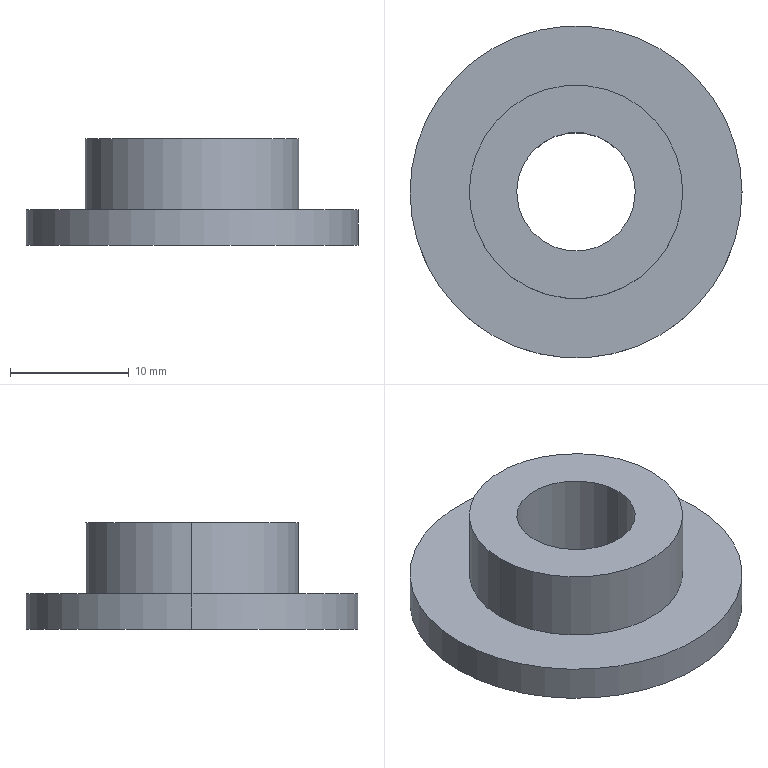Part | SolidWorks | features ICE 2, Extrusion 1 | 1 solid | 9 faces | box 28 x 28 x 9 mm | volume 2667 mm3 | cylinder 6 | plane 3 | commonest cylinder face diameters 10 x2 18 x2 28 x2
STEP:
#1=CARTESIAN_POINT('',(-5.,0.,0.));
#2=VERTEX_POINT('',#1);
#3=CARTESIAN_POINT('',(5.,0.,0.));
#4=VERTEX_POINT('',#3);
#5=CARTESIAN_POINT('',(0.,0.,0.));
#6=DIRECTION('',(0.,0.,1.));
#7=DIRECTION('',(1.,0.,0.));
#8=AXIS2_PLACEMENT_3D('',#5,#6,#7);
#9=CIRCLE('',#8,5.);
#10=EDGE_CURVE('',#2,#4,#9,.T.);
#11=ORIENTED_EDGE('',*,*,#10,.F.);
#12=CARTESIAN_POINT('',(-5.,0.,9.));
#13=VERTEX_POINT('',#12);
#14=CARTESIAN_POINT('',(-5.,0.,-3.));
#15=DIRECTION('',(0.,0.,1.));
#16=VECTOR('',#15,1000.);
#17=LINE('',#14,#16);
#18=EDGE_CURVE('',#2,#13,#17,.T.);
#19=ORIENTED_EDGE('',*,*,#18,.T.);
#20=CARTESIAN_POINT('',(5.,0.,9.));
#21=VERTEX_POINT('',#20);
#22=CARTESIAN_POINT('',(0.,0.,9.));
#23=DIRECTION('',(0.,0.,1.));
#24=DIRECTION('',(1.,0.,0.));
#25=AXIS2_PLACEMENT_3D('',#22,#23,#24);
#26=CIRCLE('',#25,5.);
#27=EDGE_CURVE('',#13,#21,#26,.T.);
#28=ORIENTED_EDGE('',*,*,#27,.T.);
#29=CARTESIAN_POINT('',(5.,0.,-3.));
#30=DIRECTION('',(0.,0.,1.));
#31=VECTOR('',#30,1000.);
#32=LINE('',#29,#31);
#33=EDGE_CURVE('',#4,#21,#32,.T.);
#34=ORIENTED_EDGE('',*,*,#33,.F.);
#35=EDGE_LOOP('',(#11,#19,#28,#34));
#36=FACE_OUTER_BOUND('',#35,.T.);
#37=CARTESIAN_POINT('',(0.,0.,-3.));
#38=DIRECTION('',(0.,0.,1.));
#39=DIRECTION('',(1.,0.,0.));
#40=AXIS2_PLACEMENT_3D('',#37,#38,#39);
#41=CYLINDRICAL_SURFACE('',#40,5.);
#42=ADVANCED_FACE('',(#36),#41,.F.);
#43=CARTESIAN_POINT('',(9.,0.,9.));
#44=VERTEX_POINT('',#43);
#45=CARTESIAN_POINT('',(-9.,0.,9.));
#46=VERTEX_POINT('',#45);
#47=CARTESIAN_POINT('',(0.,0.,9.));
#48=DIRECTION('',(0.,0.,1.));
#49=DIRECTION('',(1.,0.,0.));
#50=AXIS2_PLACEMENT_3D('',#47,#48,#49);
#51=CIRCLE('',#50,9.);
#52=EDGE_CURVE('',#44,#46,#51,.T.);
#53=ORIENTED_EDGE('',*,*,#52,.F.);
#54=CARTESIAN_POINT('',(9.,0.,3.));
#55=VERTEX_POINT('',#54);
#56=CARTESIAN_POINT('',(9.,0.,9.));
#57=DIRECTION('',(0.,0.,-1.));
#58=VECTOR('',#57,1000.);
#59=LINE('',#56,#58);
#60=EDGE_CURVE('',#44,#55,#59,.T.);
#61=ORIENTED_EDGE('',*,*,#60,.T.);
#62=CARTESIAN_POINT('',(-9.,0.,3.));
#63=VERTEX_POINT('',#62);
#64=CARTESIAN_POINT('',(0.,0.,3.));
#65=DIRECTION('',(0.,0.,1.));
#66=DIRECTION('',(1.,0.,0.));
#67=AXIS2_PLACEMENT_3D('',#64,#65,#66);
#68=CIRCLE('',#67,9.);
#69=EDGE_CURVE('',#55,#63,#68,.T.);
#70=ORIENTED_EDGE('',*,*,#69,.T.);
#71=CARTESIAN_POINT('',(-9.,0.,9.));
#72=DIRECTION('',(0.,0.,-1.));
#73=VECTOR('',#72,1000.);
#74=LINE('',#71,#73);
#75=EDGE_CURVE('',#46,#63,#74,.T.);
#76=ORIENTED_EDGE('',*,*,#75,.F.);
#77=EDGE_LOOP('',(#53,#61,#70,#76));
#78=FACE_OUTER_BOUND('',#77,.T.);
#79=CARTESIAN_POINT('',(0.,0.,9.));
#80=DIRECTION('',(0.,0.,-1.));
#81=DIRECTION('',(-1.,0.,0.));
#82=AXIS2_PLACEMENT_3D('',#79,#80,#81);
#83=CYLINDRICAL_SURFACE('',#82,9.);
#84=ADVANCED_FACE('',(#78),#83,.T.);
#85=CARTESIAN_POINT('',(14.,0.,3.));
#86=VERTEX_POINT('',#85);
#87=CARTESIAN_POINT('',(-14.,0.,3.));
#88=VERTEX_POINT('',#87);
#89=CARTESIAN_POINT('',(0.,0.,3.));
#90=DIRECTION('',(0.,0.,1.));
#91=DIRECTION('',(1.,0.,0.));
#92=AXIS2_PLACEMENT_3D('',#89,#90,#91);
#93=CIRCLE('',#92,14.);
#94=EDGE_CURVE('',#86,#88,#93,.T.);
#95=ORIENTED_EDGE('',*,*,#94,.F.);
#96=CARTESIAN_POINT('',(14.,0.,0.));
#97=VERTEX_POINT('',#96);
#98=CARTESIAN_POINT('',(14.,0.,3.));
#99=DIRECTION('',(0.,0.,-1.));
#100=VECTOR('',#99,1000.);
#101=LINE('',#98,#100);
#102=EDGE_CURVE('',#86,#97,#101,.T.);
#103=ORIENTED_EDGE('',*,*,#102,.T.);
#104=CARTESIAN_POINT('',(-14.,0.,0.));
#105=VERTEX_POINT('',#104);
#106=CARTESIAN_POINT('',(0.,0.,0.));
#107=DIRECTION('',(0.,0.,1.));
#108=DIRECTION('',(1.,0.,0.));
#109=AXIS2_PLACEMENT_3D('',#106,#107,#108);
#110=CIRCLE('',#109,14.);
#111=EDGE_CURVE('',#97,#105,#110,.T.);
#112=ORIENTED_EDGE('',*,*,#111,.T.);
#113=CARTESIAN_POINT('',(-14.,0.,3.));
#114=DIRECTION('',(0.,0.,-1.));
#115=VECTOR('',#114,1000.);
#116=LINE('',#113,#115);
#117=EDGE_CURVE('',#88,#105,#116,.T.);
#118=ORIENTED_EDGE('',*,*,#117,.F.);
#119=EDGE_LOOP('',(#95,#103,#112,#118));
#120=FACE_OUTER_BOUND('',#119,.T.);
#121=CARTESIAN_POINT('',(0.,0.,3.));
#122=DIRECTION('',(0.,0.,-1.));
#123=DIRECTION('',(-1.,0.,0.));
#124=AXIS2_PLACEMENT_3D('',#121,#122,#123);
#125=CYLINDRICAL_SURFACE('',#124,14.);
#126=ADVANCED_FACE('',(#120),#125,.T.);
#127=ORIENTED_EDGE('',*,*,#102,.F.);
#128=CARTESIAN_POINT('',(0.,0.,3.));
#129=DIRECTION('',(0.,0.,1.));
#130=DIRECTION('',(1.,0.,0.));
#131=AXIS2_PLACEMENT_3D('',#128,#129,#130);
#132=CIRCLE('',#131,14.);
#133=EDGE_CURVE('',#88,#86,#132,.T.);
#134=ORIENTED_EDGE('',*,*,#133,.F.);
#135=ORIENTED_EDGE('',*,*,#117,.T.);
#136=CARTESIAN_POINT('',(0.,0.,0.));
#137=DIRECTION('',(0.,0.,1.));
#138=DIRECTION('',(1.,0.,0.));
#139=AXIS2_PLACEMENT_3D('',#136,#137,#138);
#140=CIRCLE('',#139,14.);
#141=EDGE_CURVE('',#105,#97,#140,.T.);
#142=ORIENTED_EDGE('',*,*,#141,.T.);
#143=EDGE_LOOP('',(#127,#134,#135,#142));
#144=FACE_OUTER_BOUND('',#143,.T.);
#145=CARTESIAN_POINT('',(0.,0.,3.));
#146=DIRECTION('',(0.,0.,-1.));
#147=DIRECTION('',(-1.,0.,0.));
#148=AXIS2_PLACEMENT_3D('',#145,#146,#147);
#149=CYLINDRICAL_SURFACE('',#148,14.);
#150=ADVANCED_FACE('',(#144),#149,.T.);
#151=CARTESIAN_POINT('',(0.,0.,3.));
#152=DIRECTION('',(0.,0.,1.));
#153=DIRECTION('',(1.,0.,0.));
#154=AXIS2_PLACEMENT_3D('',#151,#152,#153);
#155=CIRCLE('',#154,9.);
#156=EDGE_CURVE('',#63,#55,#155,.T.);
#157=ORIENTED_EDGE('',*,*,#156,.F.);
#158=ORIENTED_EDGE('',*,*,#69,.F.);
#159=EDGE_LOOP('',(#157,#158));
#160=FACE_BOUND('',#159,.T.);
#161=ORIENTED_EDGE('',*,*,#133,.T.);
#162=ORIENTED_EDGE('',*,*,#94,.T.);
#163=EDGE_LOOP('',(#161,#162));
#164=FACE_OUTER_BOUND('',#163,.T.);
#165=CARTESIAN_POINT('',(0.,0.,3.));
#166=DIRECTION('',(0.,0.,1.));
#167=DIRECTION('',(1.,0.,0.));
#168=AXIS2_PLACEMENT_3D('',#165,#166,#167);
#169=PLANE('',#168);
#170=ADVANCED_FACE('',(#160,#164),#169,.T.);
#171=CARTESIAN_POINT('',(0.,0.,0.));
#172=DIRECTION('',(0.,0.,1.));
#173=DIRECTION('',(1.,0.,0.));
#174=AXIS2_PLACEMENT_3D('',#171,#172,#173);
#175=CIRCLE('',#174,5.);
#176=EDGE_CURVE('',#4,#2,#175,.T.);
#177=ORIENTED_EDGE('',*,*,#176,.T.);
#178=ORIENTED_EDGE('',*,*,#10,.T.);
#179=EDGE_LOOP('',(#177,#178));
#180=FACE_BOUND('',#179,.T.);
#181=ORIENTED_EDGE('',*,*,#141,.F.);
#182=ORIENTED_EDGE('',*,*,#111,.F.);
#183=EDGE_LOOP('',(#181,#182));
#184=FACE_OUTER_BOUND('',#183,.T.);
#185=CARTESIAN_POINT('',(0.,0.,0.));
#186=DIRECTION('',(0.,0.,1.));
#187=DIRECTION('',(1.,0.,0.));
#188=AXIS2_PLACEMENT_3D('',#185,#186,#187);
#189=PLANE('',#188);
#190=ADVANCED_FACE('',(#180,#184),#189,.F.);
#191=ORIENTED_EDGE('',*,*,#60,.F.);
#192=CARTESIAN_POINT('',(0.,0.,9.));
#193=DIRECTION('',(0.,0.,1.));
#194=DIRECTION('',(1.,0.,0.));
#195=AXIS2_PLACEMENT_3D('',#192,#193,#194);
#196=CIRCLE('',#195,9.);
#197=EDGE_CURVE('',#46,#44,#196,.T.);
#198=ORIENTED_EDGE('',*,*,#197,.F.);
#199=ORIENTED_EDGE('',*,*,#75,.T.);
#200=ORIENTED_EDGE('',*,*,#156,.T.);
#201=EDGE_LOOP('',(#191,#198,#199,#200));
#202=FACE_OUTER_BOUND('',#201,.T.);
#203=CARTESIAN_POINT('',(0.,0.,9.));
#204=DIRECTION('',(0.,0.,-1.));
#205=DIRECTION('',(-1.,0.,0.));
#206=AXIS2_PLACEMENT_3D('',#203,#204,#205);
#207=CYLINDRICAL_SURFACE('',#206,9.);
#208=ADVANCED_FACE('',(#202),#207,.T.);
#209=CARTESIAN_POINT('',(0.,0.,9.));
#210=DIRECTION('',(0.,0.,1.));
#211=DIRECTION('',(1.,0.,0.));
#212=AXIS2_PLACEMENT_3D('',#209,#210,#211);
#213=CIRCLE('',#212,5.);
#214=EDGE_CURVE('',#21,#13,#213,.T.);
#215=ORIENTED_EDGE('',*,*,#214,.F.);
#216=ORIENTED_EDGE('',*,*,#27,.F.);
#217=EDGE_LOOP('',(#215,#216));
#218=FACE_BOUND('',#217,.T.);
#219=ORIENTED_EDGE('',*,*,#197,.T.);
#220=ORIENTED_EDGE('',*,*,#52,.T.);
#221=EDGE_LOOP('',(#219,#220));
#222=FACE_OUTER_BOUND('',#221,.T.);
#223=CARTESIAN_POINT('',(0.,0.,9.));
#224=DIRECTION('',(0.,0.,1.));
#225=DIRECTION('',(1.,0.,0.));
#226=AXIS2_PLACEMENT_3D('',#223,#224,#225);
#227=PLANE('',#226);
#228=ADVANCED_FACE('',(#218,#222),#227,.T.);
#229=ORIENTED_EDGE('',*,*,#18,.F.);
#230=ORIENTED_EDGE('',*,*,#176,.F.);
#231=ORIENTED_EDGE('',*,*,#33,.T.);
#232=ORIENTED_EDGE('',*,*,#214,.T.);
#233=EDGE_LOOP('',(#229,#230,#231,#232));
#234=FACE_OUTER_BOUND('',#233,.T.);
#235=CARTESIAN_POINT('',(0.,0.,-3.));
#236=DIRECTION('',(0.,0.,1.));
#237=DIRECTION('',(1.,0.,0.));
#238=AXIS2_PLACEMENT_3D('',#235,#236,#237);
#239=CYLINDRICAL_SURFACE('',#238,5.);
#240=ADVANCED_FACE('',(#234),#239,.F.);
#241=CLOSED_SHELL('',(#42,#84,#126,#150,#170,#190,#208,#228,#240));
#242=MANIFOLD_SOLID_BREP('',#241);
#243=CARTESIAN_POINT('',(0.,0.,0.));
#244=DIRECTION('',(0.,0.,1.));
#245=DIRECTION('',(1.,0.,0.));
#246=AXIS2_PLACEMENT_3D('',#243,#244,#245);
#247=(LENGTH_UNIT()NAMED_UNIT(*)SI_UNIT(.MILLI.,.METRE.));
#248=UNCERTAINTY_MEASURE_WITH_UNIT(LENGTH_MEASURE(0.00001),#247,'','');
#249=(NAMED_UNIT(*)PLANE_ANGLE_UNIT()SI_UNIT($,.RADIAN.));
#250=(NAMED_UNIT(*)SI_UNIT($,.STERADIAN.)SOLID_ANGLE_UNIT());
#251=(GEOMETRIC_REPRESENTATION_CONTEXT(3)GLOBAL_UNCERTAINTY_ASSIGNED_CONTEXT((#248))GLOBAL_UNIT_ASSIGNED_CONTEXT((#247,#249,#250))REPRESENTATION_CONTEXT('',''));
#252=ADVANCED_BREP_SHAPE_REPRESENTATION('',(#242,#246),#251);